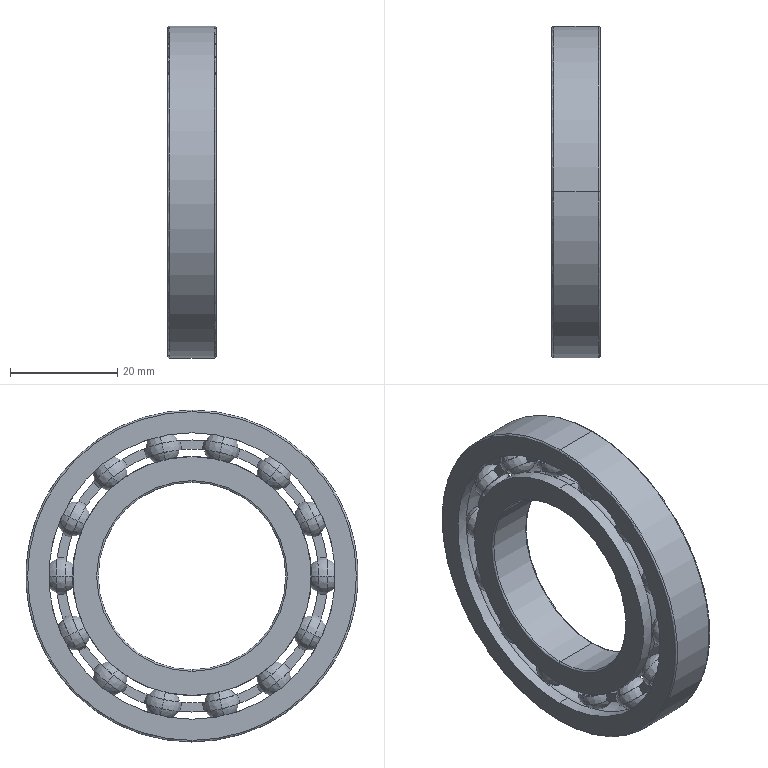Part | SolidWorks | features Revolution 5, CirPattern 2, RevCut 2 | 1 solid | 213 faces | box 9 x 62 x 62 mm | volume 13612 mm3 | sphere 112 | torus 53 | plane 32 | cylinder 16 | commonest cylinder face diameters 44.6 x4 53.5 x4 35 x2 47.304 x2 50.796 x2 62 x2